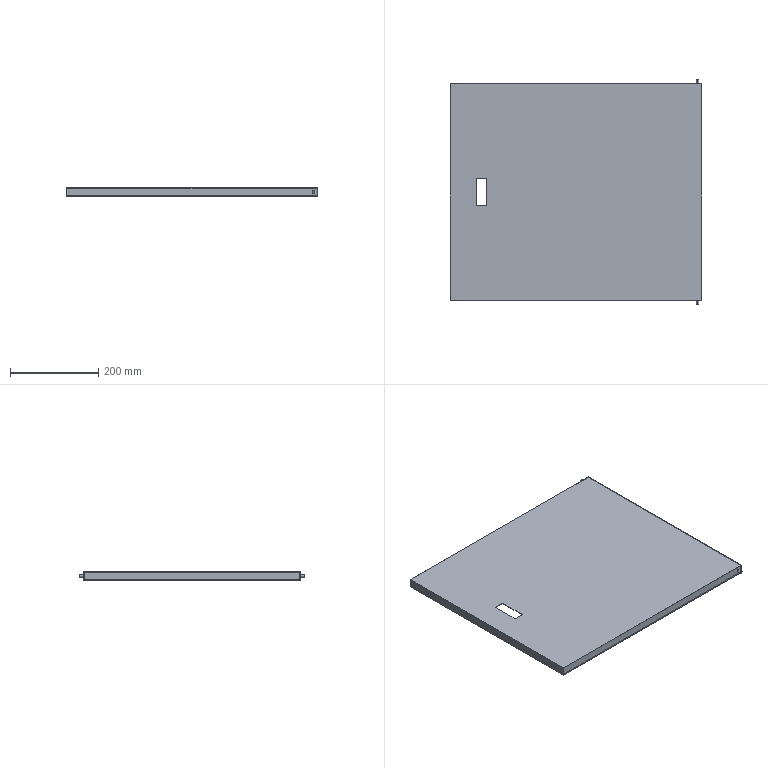Part | SolidWorks | features ICE 4, Extrusion 1, Shell 1 | 1 solid | 26 faces | box 570 x 510 x 20 mm | volume 346646 mm3 | plane 22 | cylinder 4 | commonest cylinder face diameters 6 x4
STEP:
#1=CARTESIAN_POINT('',(275.,-255.,7.));
#2=VERTEX_POINT('',#1);
#3=CARTESIAN_POINT('',(275.,-255.,13.));
#4=VERTEX_POINT('',#3);
#5=CARTESIAN_POINT('',(275.,-255.,10.));
#6=DIRECTION('',(0.,-1.,0.));
#7=DIRECTION('',(0.,0.,-1.));
#8=AXIS2_PLACEMENT_3D('',#5,#6,#7);
#9=CIRCLE('',#8,3.);
#10=EDGE_CURVE('',#2,#4,#9,.T.);
#11=ORIENTED_EDGE('',*,*,#10,.F.);
#12=CARTESIAN_POINT('',(275.,-245.,7.));
#13=VERTEX_POINT('',#12);
#14=CARTESIAN_POINT('',(275.,-255.,7.));
#15=DIRECTION('',(0.,1.,0.));
#16=VECTOR('',#15,1000.);
#17=LINE('',#14,#16);
#18=EDGE_CURVE('',#2,#13,#17,.T.);
#19=ORIENTED_EDGE('',*,*,#18,.T.);
#20=CARTESIAN_POINT('',(275.,-245.,13.));
#21=VERTEX_POINT('',#20);
#22=CARTESIAN_POINT('',(275.,-245.,10.));
#23=DIRECTION('',(0.,-1.,0.));
#24=DIRECTION('',(0.,0.,1.));
#25=AXIS2_PLACEMENT_3D('',#22,#23,#24);
#26=CIRCLE('',#25,3.);
#27=EDGE_CURVE('',#13,#21,#26,.T.);
#28=ORIENTED_EDGE('',*,*,#27,.T.);
#29=CARTESIAN_POINT('',(275.,-255.,13.));
#30=DIRECTION('',(0.,1.,0.));
#31=VECTOR('',#30,1000.);
#32=LINE('',#29,#31);
#33=EDGE_CURVE('',#4,#21,#32,.T.);
#34=ORIENTED_EDGE('',*,*,#33,.F.);
#35=EDGE_LOOP('',(#11,#19,#28,#34));
#36=FACE_OUTER_BOUND('',#35,.T.);
#37=CARTESIAN_POINT('',(275.,-255.,10.));
#38=DIRECTION('',(0.,1.,0.));
#39=DIRECTION('',(0.,0.,1.));
#40=AXIS2_PLACEMENT_3D('',#37,#38,#39);
#41=CYLINDRICAL_SURFACE('',#40,3.);
#42=ADVANCED_FACE('',(#36),#41,.T.);
#43=CARTESIAN_POINT('',(275.,255.,13.));
#44=VERTEX_POINT('',#43);
#45=CARTESIAN_POINT('',(275.,255.,7.));
#46=VERTEX_POINT('',#45);
#47=CARTESIAN_POINT('',(275.,255.,10.));
#48=DIRECTION('',(0.,1.,0.));
#49=DIRECTION('',(0.,0.,1.));
#50=AXIS2_PLACEMENT_3D('',#47,#48,#49);
#51=CIRCLE('',#50,3.);
#52=EDGE_CURVE('',#44,#46,#51,.T.);
#53=ORIENTED_EDGE('',*,*,#52,.F.);
#54=CARTESIAN_POINT('',(275.,245.,13.));
#55=VERTEX_POINT('',#54);
#56=CARTESIAN_POINT('',(275.,255.,13.));
#57=DIRECTION('',(0.,-1.,0.));
#58=VECTOR('',#57,1000.);
#59=LINE('',#56,#58);
#60=EDGE_CURVE('',#44,#55,#59,.T.);
#61=ORIENTED_EDGE('',*,*,#60,.T.);
#62=CARTESIAN_POINT('',(275.,245.,7.));
#63=VERTEX_POINT('',#62);
#64=CARTESIAN_POINT('',(275.,245.,10.));
#65=DIRECTION('',(0.,1.,0.));
#66=DIRECTION('',(0.,0.,-1.));
#67=AXIS2_PLACEMENT_3D('',#64,#65,#66);
#68=CIRCLE('',#67,3.);
#69=EDGE_CURVE('',#55,#63,#68,.T.);
#70=ORIENTED_EDGE('',*,*,#69,.T.);
#71=CARTESIAN_POINT('',(275.,255.,7.));
#72=DIRECTION('',(0.,-1.,0.));
#73=VECTOR('',#72,1000.);
#74=LINE('',#71,#73);
#75=EDGE_CURVE('',#46,#63,#74,.T.);
#76=ORIENTED_EDGE('',*,*,#75,.F.);
#77=EDGE_LOOP('',(#53,#61,#70,#76));
#78=FACE_OUTER_BOUND('',#77,.T.);
#79=CARTESIAN_POINT('',(275.,255.,10.));
#80=DIRECTION('',(0.,-1.,0.));
#81=DIRECTION('',(0.,0.,-1.));
#82=AXIS2_PLACEMENT_3D('',#79,#80,#81);
#83=CYLINDRICAL_SURFACE('',#82,3.);
#84=ADVANCED_FACE('',(#78),#83,.T.);
#85=CARTESIAN_POINT('',(-285.,-245.,0.));
#86=VERTEX_POINT('',#85);
#87=CARTESIAN_POINT('',(285.,-245.,0.));
#88=VERTEX_POINT('',#87);
#89=CARTESIAN_POINT('',(-285.,-245.,0.));
#90=DIRECTION('',(1.,0.,0.));
#91=VECTOR('',#90,1000.);
#92=LINE('',#89,#91);
#93=EDGE_CURVE('',#86,#88,#92,.T.);
#94=ORIENTED_EDGE('',*,*,#93,.T.);
#95=CARTESIAN_POINT('',(285.,-245.,20.));
#96=VERTEX_POINT('',#95);
#97=CARTESIAN_POINT('',(285.,-245.,20.));
#98=DIRECTION('',(0.,0.,-1.));
#99=VECTOR('',#98,1000.);
#100=LINE('',#97,#99);
#101=EDGE_CURVE('',#96,#88,#100,.T.);
#102=ORIENTED_EDGE('',*,*,#101,.F.);
#103=CARTESIAN_POINT('',(-285.,-245.,20.));
#104=VERTEX_POINT('',#103);
#105=CARTESIAN_POINT('',(-285.,-245.,20.));
#106=DIRECTION('',(1.,0.,0.));
#107=VECTOR('',#106,1000.);
#108=LINE('',#105,#107);
#109=EDGE_CURVE('',#104,#96,#108,.T.);
#110=ORIENTED_EDGE('',*,*,#109,.F.);
#111=CARTESIAN_POINT('',(-285.,-245.,20.));
#112=DIRECTION('',(0.,0.,-1.));
#113=VECTOR('',#112,1000.);
#114=LINE('',#111,#113);
#115=EDGE_CURVE('',#104,#86,#114,.T.);
#116=ORIENTED_EDGE('',*,*,#115,.T.);
#117=EDGE_LOOP('',(#94,#102,#110,#116));
#118=FACE_OUTER_BOUND('',#117,.T.);
#119=CARTESIAN_POINT('',(275.,-245.,10.));
#120=DIRECTION('',(0.,-1.,0.));
#121=DIRECTION('',(0.,0.,1.));
#122=AXIS2_PLACEMENT_3D('',#119,#120,#121);
#123=CIRCLE('',#122,3.);
#124=EDGE_CURVE('',#21,#13,#123,.T.);
#125=ORIENTED_EDGE('',*,*,#124,.F.);
#126=ORIENTED_EDGE('',*,*,#27,.F.);
#127=EDGE_LOOP('',(#125,#126));
#128=FACE_BOUND('',#127,.T.);
#129=CARTESIAN_POINT('',(-285.,-245.,20.));
#130=DIRECTION('',(0.,1.,0.));
#131=DIRECTION('',(0.,0.,1.));
#132=AXIS2_PLACEMENT_3D('',#129,#130,#131);
#133=PLANE('',#132);
#134=ADVANCED_FACE('',(#118,#128),#133,.F.);
#135=CARTESIAN_POINT('',(285.,245.,0.));
#136=VERTEX_POINT('',#135);
#137=CARTESIAN_POINT('',(-285.,245.,0.));
#138=VERTEX_POINT('',#137);
#139=CARTESIAN_POINT('',(-285.,245.,0.));
#140=DIRECTION('',(-1.,0.,0.));
#141=VECTOR('',#140,1000.);
#142=LINE('',#139,#141);
#143=EDGE_CURVE('',#136,#138,#142,.T.);
#144=ORIENTED_EDGE('',*,*,#143,.T.);
#145=CARTESIAN_POINT('',(-285.,245.,20.));
#146=VERTEX_POINT('',#145);
#147=CARTESIAN_POINT('',(-285.,245.,20.));
#148=DIRECTION('',(0.,0.,-1.));
#149=VECTOR('',#148,1000.);
#150=LINE('',#147,#149);
#151=EDGE_CURVE('',#146,#138,#150,.T.);
#152=ORIENTED_EDGE('',*,*,#151,.F.);
#153=CARTESIAN_POINT('',(285.,245.,20.));
#154=VERTEX_POINT('',#153);
#155=CARTESIAN_POINT('',(-285.,245.,20.));
#156=DIRECTION('',(-1.,0.,0.));
#157=VECTOR('',#156,1000.);
#158=LINE('',#155,#157);
#159=EDGE_CURVE('',#154,#146,#158,.T.);
#160=ORIENTED_EDGE('',*,*,#159,.F.);
#161=CARTESIAN_POINT('',(285.,245.,20.));
#162=DIRECTION('',(0.,0.,-1.));
#163=VECTOR('',#162,1000.);
#164=LINE('',#161,#163);
#165=EDGE_CURVE('',#154,#136,#164,.T.);
#166=ORIENTED_EDGE('',*,*,#165,.T.);
#167=EDGE_LOOP('',(#144,#152,#160,#166));
#168=FACE_OUTER_BOUND('',#167,.T.);
#169=CARTESIAN_POINT('',(275.,245.,10.));
#170=DIRECTION('',(0.,1.,0.));
#171=DIRECTION('',(0.,0.,-1.));
#172=AXIS2_PLACEMENT_3D('',#169,#170,#171);
#173=CIRCLE('',#172,3.);
#174=EDGE_CURVE('',#63,#55,#173,.T.);
#175=ORIENTED_EDGE('',*,*,#174,.F.);
#176=ORIENTED_EDGE('',*,*,#69,.F.);
#177=EDGE_LOOP('',(#175,#176));
#178=FACE_BOUND('',#177,.T.);
#179=CARTESIAN_POINT('',(-285.,245.,20.));
#180=DIRECTION('',(0.,-1.,0.));
#181=DIRECTION('',(0.,0.,-1.));
#182=AXIS2_PLACEMENT_3D('',#179,#180,#181);
#183=PLANE('',#182);
#184=ADVANCED_FACE('',(#168,#178),#183,.F.);
#185=CARTESIAN_POINT('',(285.,245.,0.));
#186=DIRECTION('',(0.,1.,0.));
#187=VECTOR('',#186,1000.);
#188=LINE('',#185,#187);
#189=EDGE_CURVE('',#88,#136,#188,.T.);
#190=ORIENTED_EDGE('',*,*,#189,.T.);
#191=ORIENTED_EDGE('',*,*,#165,.F.);
#192=CARTESIAN_POINT('',(285.,245.,20.));
#193=DIRECTION('',(0.,1.,0.));
#194=VECTOR('',#193,1000.);
#195=LINE('',#192,#194);
#196=EDGE_CURVE('',#96,#154,#195,.T.);
#197=ORIENTED_EDGE('',*,*,#196,.F.);
#198=ORIENTED_EDGE('',*,*,#101,.T.);
#199=EDGE_LOOP('',(#190,#191,#197,#198));
#200=FACE_OUTER_BOUND('',#199,.T.);
#201=CARTESIAN_POINT('',(285.,245.,20.));
#202=DIRECTION('',(-1.,0.,0.));
#203=DIRECTION('',(0.,0.,1.));
#204=AXIS2_PLACEMENT_3D('',#201,#202,#203);
#205=PLANE('',#204);
#206=ADVANCED_FACE('',(#200),#205,.F.);
#207=CARTESIAN_POINT('',(-285.,245.,0.));
#208=DIRECTION('',(0.,-1.,0.));
#209=VECTOR('',#208,1000.);
#210=LINE('',#207,#209);
#211=EDGE_CURVE('',#138,#86,#210,.T.);
#212=ORIENTED_EDGE('',*,*,#211,.T.);
#213=ORIENTED_EDGE('',*,*,#115,.F.);
#214=CARTESIAN_POINT('',(-285.,245.,20.));
#215=DIRECTION('',(0.,-1.,0.));
#216=VECTOR('',#215,1000.);
#217=LINE('',#214,#216);
#218=EDGE_CURVE('',#146,#104,#217,.T.);
#219=ORIENTED_EDGE('',*,*,#218,.F.);
#220=ORIENTED_EDGE('',*,*,#151,.T.);
#221=EDGE_LOOP('',(#212,#213,#219,#220));
#222=FACE_OUTER_BOUND('',#221,.T.);
#223=CARTESIAN_POINT('',(-285.,245.,20.));
#224=DIRECTION('',(1.,0.,0.));
#225=DIRECTION('',(0.,0.,-1.));
#226=AXIS2_PLACEMENT_3D('',#223,#224,#225);
#227=PLANE('',#226);
#228=ADVANCED_FACE('',(#222),#227,.F.);
#229=CARTESIAN_POINT('',(-202.,-31.5,20.));
#230=VERTEX_POINT('',#229);
#231=CARTESIAN_POINT('',(-202.,31.5,20.));
#232=VERTEX_POINT('',#231);
#233=CARTESIAN_POINT('',(-202.,-31.5,20.));
#234=DIRECTION('',(0.,1.,0.));
#235=VECTOR('',#234,1000.);
#236=LINE('',#233,#235);
#237=EDGE_CURVE('',#230,#232,#236,.T.);
#238=ORIENTED_EDGE('',*,*,#237,.F.);
#239=CARTESIAN_POINT('',(-225.,-31.5,20.));
#240=VERTEX_POINT('',#239);
#241=CARTESIAN_POINT('',(-225.,-31.5,20.));
#242=DIRECTION('',(1.,0.,0.));
#243=VECTOR('',#242,1000.);
#244=LINE('',#241,#243);
#245=EDGE_CURVE('',#240,#230,#244,.T.);
#246=ORIENTED_EDGE('',*,*,#245,.F.);
#247=CARTESIAN_POINT('',(-225.,31.5,20.));
#248=VERTEX_POINT('',#247);
#249=CARTESIAN_POINT('',(-225.,-31.5,20.));
#250=DIRECTION('',(0.,-1.,0.));
#251=VECTOR('',#250,1000.);
#252=LINE('',#249,#251);
#253=EDGE_CURVE('',#248,#240,#252,.T.);
#254=ORIENTED_EDGE('',*,*,#253,.F.);
#255=CARTESIAN_POINT('',(-225.,31.5,20.));
#256=DIRECTION('',(-1.,0.,0.));
#257=VECTOR('',#256,1000.);
#258=LINE('',#255,#257);
#259=EDGE_CURVE('',#232,#248,#258,.T.);
#260=ORIENTED_EDGE('',*,*,#259,.F.);
#261=EDGE_LOOP('',(#238,#246,#254,#260));
#262=FACE_BOUND('',#261,.T.);
#263=ORIENTED_EDGE('',*,*,#196,.T.);
#264=ORIENTED_EDGE('',*,*,#159,.T.);
#265=ORIENTED_EDGE('',*,*,#218,.T.);
#266=ORIENTED_EDGE('',*,*,#109,.T.);
#267=EDGE_LOOP('',(#263,#264,#265,#266));
#268=FACE_OUTER_BOUND('',#267,.T.);
#269=CARTESIAN_POINT('',(285.,-245.,20.));
#270=DIRECTION('',(0.,0.,1.));
#271=DIRECTION('',(1.,0.,0.));
#272=AXIS2_PLACEMENT_3D('',#269,#270,#271);
#273=PLANE('',#272);
#274=ADVANCED_FACE('',(#262,#268),#273,.T.);
#275=ORIENTED_EDGE('',*,*,#189,.F.);
#276=ORIENTED_EDGE('',*,*,#93,.F.);
#277=ORIENTED_EDGE('',*,*,#211,.F.);
#278=ORIENTED_EDGE('',*,*,#143,.F.);
#279=EDGE_LOOP('',(#275,#276,#277,#278));
#280=FACE_OUTER_BOUND('',#279,.T.);
#281=CARTESIAN_POINT('',(-275.,235.,0.));
#282=VERTEX_POINT('',#281);
#283=CARTESIAN_POINT('',(275.,235.,0.));
#284=VERTEX_POINT('',#283);
#285=CARTESIAN_POINT('',(275.,235.,0.));
#286=DIRECTION('',(1.,0.,0.));
#287=VECTOR('',#286,1000.);
#288=LINE('',#285,#287);
#289=EDGE_CURVE('',#282,#284,#288,.T.);
#290=ORIENTED_EDGE('',*,*,#289,.F.);
#291=CARTESIAN_POINT('',(-275.,-235.,0.));
#292=VERTEX_POINT('',#291);
#293=CARTESIAN_POINT('',(-275.,235.,0.));
#294=DIRECTION('',(0.,1.,0.));
#295=VECTOR('',#294,1000.);
#296=LINE('',#293,#295);
#297=EDGE_CURVE('',#292,#282,#296,.T.);
#298=ORIENTED_EDGE('',*,*,#297,.F.);
#299=CARTESIAN_POINT('',(275.,-235.,0.));
#300=VERTEX_POINT('',#299);
#301=CARTESIAN_POINT('',(275.,-235.,0.));
#302=DIRECTION('',(-1.,0.,0.));
#303=VECTOR('',#302,1000.);
#304=LINE('',#301,#303);
#305=EDGE_CURVE('',#300,#292,#304,.T.);
#306=ORIENTED_EDGE('',*,*,#305,.F.);
#307=CARTESIAN_POINT('',(275.,235.,0.));
#308=DIRECTION('',(0.,-1.,0.));
#309=VECTOR('',#308,1000.);
#310=LINE('',#307,#309);
#311=EDGE_CURVE('',#284,#300,#310,.T.);
#312=ORIENTED_EDGE('',*,*,#311,.F.);
#313=EDGE_LOOP('',(#290,#298,#306,#312));
#314=FACE_BOUND('',#313,.T.);
#315=CARTESIAN_POINT('',(285.,-245.,0.));
#316=DIRECTION('',(0.,0.,1.));
#317=DIRECTION('',(1.,0.,0.));
#318=AXIS2_PLACEMENT_3D('',#315,#316,#317);
#319=PLANE('',#318);
#320=ADVANCED_FACE('',(#280,#314),#319,.F.);
#321=CARTESIAN_POINT('',(284.,244.,1.5));
#322=VERTEX_POINT('',#321);
#323=CARTESIAN_POINT('',(284.,-244.,1.5));
#324=VERTEX_POINT('',#323);
#325=CARTESIAN_POINT('',(284.,245.,1.5));
#326=DIRECTION('',(0.,-1.,0.));
#327=VECTOR('',#326,1000.);
#328=LINE('',#325,#327);
#329=EDGE_CURVE('',#322,#324,#328,.T.);
#330=ORIENTED_EDGE('',*,*,#329,.F.);
#331=CARTESIAN_POINT('',(-284.,244.,1.5));
#332=VERTEX_POINT('',#331);
#333=CARTESIAN_POINT('',(-285.,244.,1.5));
#334=DIRECTION('',(1.,0.,0.));
#335=VECTOR('',#334,1000.);
#336=LINE('',#333,#335);
#337=EDGE_CURVE('',#332,#322,#336,.T.);
#338=ORIENTED_EDGE('',*,*,#337,.F.);
#339=CARTESIAN_POINT('',(-284.,-244.,1.5));
#340=VERTEX_POINT('',#339);
#341=CARTESIAN_POINT('',(-284.,245.,1.5));
#342=DIRECTION('',(0.,1.,0.));
#343=VECTOR('',#342,1000.);
#344=LINE('',#341,#343);
#345=EDGE_CURVE('',#340,#332,#344,.T.);
#346=ORIENTED_EDGE('',*,*,#345,.F.);
#347=CARTESIAN_POINT('',(-285.,-244.,1.5));
#348=DIRECTION('',(-1.,0.,0.));
#349=VECTOR('',#348,1000.);
#350=LINE('',#347,#349);
#351=EDGE_CURVE('',#324,#340,#350,.T.);
#352=ORIENTED_EDGE('',*,*,#351,.F.);
#353=EDGE_LOOP('',(#330,#338,#346,#352));
#354=FACE_OUTER_BOUND('',#353,.T.);
#355=CARTESIAN_POINT('',(-275.,-235.,1.5));
#356=VERTEX_POINT('',#355);
#357=CARTESIAN_POINT('',(-275.,235.,1.5));
#358=VERTEX_POINT('',#357);
#359=CARTESIAN_POINT('',(-275.,235.,1.5));
#360=DIRECTION('',(0.,1.,0.));
#361=VECTOR('',#360,1000.);
#362=LINE('',#359,#361);
#363=EDGE_CURVE('',#356,#358,#362,.T.);
#364=ORIENTED_EDGE('',*,*,#363,.T.);
#365=CARTESIAN_POINT('',(275.,235.,1.5));
#366=VERTEX_POINT('',#365);
#367=CARTESIAN_POINT('',(275.,235.,1.5));
#368=DIRECTION('',(1.,0.,0.));
#369=VECTOR('',#368,1000.);
#370=LINE('',#367,#369);
#371=EDGE_CURVE('',#358,#366,#370,.T.);
#372=ORIENTED_EDGE('',*,*,#371,.T.);
#373=CARTESIAN_POINT('',(275.,-235.,1.5));
#374=VERTEX_POINT('',#373);
#375=CARTESIAN_POINT('',(275.,235.,1.5));
#376=DIRECTION('',(0.,-1.,0.));
#377=VECTOR('',#376,1000.);
#378=LINE('',#375,#377);
#379=EDGE_CURVE('',#366,#374,#378,.T.);
#380=ORIENTED_EDGE('',*,*,#379,.T.);
#381=CARTESIAN_POINT('',(275.,-235.,1.5));
#382=DIRECTION('',(-1.,0.,0.));
#383=VECTOR('',#382,1000.);
#384=LINE('',#381,#383);
#385=EDGE_CURVE('',#374,#356,#384,.T.);
#386=ORIENTED_EDGE('',*,*,#385,.T.);
#387=EDGE_LOOP('',(#364,#372,#380,#386));
#388=FACE_BOUND('',#387,.T.);
#389=CARTESIAN_POINT('',(285.,-245.,1.5));
#390=DIRECTION('',(0.,0.,-1.));
#391=DIRECTION('',(-1.,0.,0.));
#392=AXIS2_PLACEMENT_3D('',#389,#390,#391);
#393=PLANE('',#392);
#394=ADVANCED_FACE('',(#354,#388),#393,.F.);
#395=ORIENTED_EDGE('',*,*,#289,.T.);
#396=CARTESIAN_POINT('',(275.,235.,1.5));
#397=DIRECTION('',(0.,0.,-1.));
#398=VECTOR('',#397,1000.);
#399=LINE('',#396,#398);
#400=EDGE_CURVE('',#366,#284,#399,.T.);
#401=ORIENTED_EDGE('',*,*,#400,.F.);
#402=ORIENTED_EDGE('',*,*,#371,.F.);
#403=CARTESIAN_POINT('',(-275.,235.,1.5));
#404=DIRECTION('',(0.,0.,-1.));
#405=VECTOR('',#404,1000.);
#406=LINE('',#403,#405);
#407=EDGE_CURVE('',#358,#282,#406,.T.);
#408=ORIENTED_EDGE('',*,*,#407,.T.);
#409=EDGE_LOOP('',(#395,#401,#402,#408));
#410=FACE_OUTER_BOUND('',#409,.T.);
#411=CARTESIAN_POINT('',(275.,235.,1.5));
#412=DIRECTION('',(0.,1.,0.));
#413=DIRECTION('',(0.,0.,1.));
#414=AXIS2_PLACEMENT_3D('',#411,#412,#413);
#415=PLANE('',#414);
#416=ADVANCED_FACE('',(#410),#415,.F.);
#417=ORIENTED_EDGE('',*,*,#297,.T.);
#418=ORIENTED_EDGE('',*,*,#407,.F.);
#419=ORIENTED_EDGE('',*,*,#363,.F.);
#420=CARTESIAN_POINT('',(-275.,-235.,1.5));
#421=DIRECTION('',(0.,0.,-1.));
#422=VECTOR('',#421,1000.);
#423=LINE('',#420,#422);
#424=EDGE_CURVE('',#356,#292,#423,.T.);
#425=ORIENTED_EDGE('',*,*,#424,.T.);
#426=EDGE_LOOP('',(#417,#418,#419,#425));
#427=FACE_OUTER_BOUND('',#426,.T.);
#428=CARTESIAN_POINT('',(-275.,235.,1.5));
#429=DIRECTION('',(-1.,0.,0.));
#430=DIRECTION('',(0.,-1.,0.));
#431=AXIS2_PLACEMENT_3D('',#428,#429,#430);
#432=PLANE('',#431);
#433=ADVANCED_FACE('',(#427),#432,.F.);
#434=ORIENTED_EDGE('',*,*,#305,.T.);
#435=ORIENTED_EDGE('',*,*,#424,.F.);
#436=ORIENTED_EDGE('',*,*,#385,.F.);
#437=CARTESIAN_POINT('',(275.,-235.,1.5));
#438=DIRECTION('',(0.,0.,-1.));
#439=VECTOR('',#438,1000.);
#440=LINE('',#437,#439);
#441=EDGE_CURVE('',#374,#300,#440,.T.);
#442=ORIENTED_EDGE('',*,*,#441,.T.);
#443=EDGE_LOOP('',(#434,#435,#436,#442));
#444=FACE_OUTER_BOUND('',#443,.T.);
#445=CARTESIAN_POINT('',(275.,-235.,1.5));
#446=DIRECTION('',(0.,-1.,0.));
#447=DIRECTION('',(1.,0.,0.));
#448=AXIS2_PLACEMENT_3D('',#445,#446,#447);
#449=PLANE('',#448);
#450=ADVANCED_FACE('',(#444),#449,.F.);
#451=ORIENTED_EDGE('',*,*,#311,.T.);
#452=ORIENTED_EDGE('',*,*,#441,.F.);
#453=ORIENTED_EDGE('',*,*,#379,.F.);
#454=ORIENTED_EDGE('',*,*,#400,.T.);
#455=EDGE_LOOP('',(#451,#452,#453,#454));
#456=FACE_OUTER_BOUND('',#455,.T.);
#457=CARTESIAN_POINT('',(275.,235.,1.5));
#458=DIRECTION('',(1.,0.,0.));
#459=DIRECTION('',(0.,1.,0.));
#460=AXIS2_PLACEMENT_3D('',#457,#458,#459);
#461=PLANE('',#460);
#462=ADVANCED_FACE('',(#456),#461,.F.);
#463=CARTESIAN_POINT('',(-225.,-31.5,19.));
#464=VERTEX_POINT('',#463);
#465=CARTESIAN_POINT('',(-202.,-31.5,19.));
#466=VERTEX_POINT('',#465);
#467=CARTESIAN_POINT('',(285.,-31.5,19.));
#468=DIRECTION('',(1.,0.,0.));
#469=VECTOR('',#468,1000.);
#470=LINE('',#467,#469);
#471=EDGE_CURVE('',#464,#466,#470,.T.);
#472=ORIENTED_EDGE('',*,*,#471,.T.);
#473=CARTESIAN_POINT('',(-202.,31.5,19.));
#474=VERTEX_POINT('',#473);
#475=CARTESIAN_POINT('',(-202.,-245.,19.));
#476=DIRECTION('',(0.,1.,0.));
#477=VECTOR('',#476,1000.);
#478=LINE('',#475,#477);
#479=EDGE_CURVE('',#466,#474,#478,.T.);
#480=ORIENTED_EDGE('',*,*,#479,.T.);
#481=CARTESIAN_POINT('',(-225.,31.5,19.));
#482=VERTEX_POINT('',#481);
#483=CARTESIAN_POINT('',(285.,31.5,19.));
#484=DIRECTION('',(-1.,0.,0.));
#485=VECTOR('',#484,1000.);
#486=LINE('',#483,#485);
#487=EDGE_CURVE('',#474,#482,#486,.T.);
#488=ORIENTED_EDGE('',*,*,#487,.T.);
#489=CARTESIAN_POINT('',(-225.,-245.,19.));
#490=DIRECTION('',(0.,-1.,0.));
#491=VECTOR('',#490,1000.);
#492=LINE('',#489,#491);
#493=EDGE_CURVE('',#482,#464,#492,.T.);
#494=ORIENTED_EDGE('',*,*,#493,.T.);
#495=EDGE_LOOP('',(#472,#480,#488,#494));
#496=FACE_BOUND('',#495,.T.);
#497=CARTESIAN_POINT('',(284.,-244.,19.));
#498=VERTEX_POINT('',#497);
#499=CARTESIAN_POINT('',(284.,244.,19.));
#500=VERTEX_POINT('',#499);
#501=CARTESIAN_POINT('',(284.,245.,19.));
#502=DIRECTION('',(0.,1.,0.));
#503=VECTOR('',#502,1000.);
#504=LINE('',#501,#503);
#505=EDGE_CURVE('',#498,#500,#504,.T.);
#506=ORIENTED_EDGE('',*,*,#505,.F.);
#507=CARTESIAN_POINT('',(-284.,-244.,19.));
#508=VERTEX_POINT('',#507);
#509=CARTESIAN_POINT('',(-285.,-244.,19.));
#510=DIRECTION('',(1.,0.,0.));
#511=VECTOR('',#510,1000.);
#512=LINE('',#509,#511);
#513=EDGE_CURVE('',#508,#498,#512,.T.);
#514=ORIENTED_EDGE('',*,*,#513,.F.);
#515=CARTESIAN_POINT('',(-284.,244.,19.));
#516=VERTEX_POINT('',#515);
#517=CARTESIAN_POINT('',(-284.,245.,19.));
#518=DIRECTION('',(0.,-1.,0.));
#519=VECTOR('',#518,1000.);
#520=LINE('',#517,#519);
#521=EDGE_CURVE('',#516,#508,#520,.T.);
#522=ORIENTED_EDGE('',*,*,#521,.F.);
#523=CARTESIAN_POINT('',(-285.,244.,19.));
#524=DIRECTION('',(-1.,0.,0.));
#525=VECTOR('',#524,1000.);
#526=LINE('',#523,#525);
#527=EDGE_CURVE('',#500,#516,#526,.T.);
#528=ORIENTED_EDGE('',*,*,#527,.F.);
#529=EDGE_LOOP('',(#506,#514,#522,#528));
#530=FACE_OUTER_BOUND('',#529,.T.);
#531=CARTESIAN_POINT('',(285.,-245.,19.));
#532=DIRECTION('',(0.,0.,1.));
#533=DIRECTION('',(1.,0.,0.));
#534=AXIS2_PLACEMENT_3D('',#531,#532,#533);
#535=PLANE('',#534);
#536=ADVANCED_FACE('',(#496,#530),#535,.F.);
#537=CARTESIAN_POINT('',(284.,-244.,20.));
#538=DIRECTION('',(0.,0.,-1.));
#539=VECTOR('',#538,1000.);
#540=LINE('',#537,#539);
#541=EDGE_CURVE('',#498,#324,#540,.T.);
#542=ORIENTED_EDGE('',*,*,#541,.T.);
#543=ORIENTED_EDGE('',*,*,#351,.T.);
#544=CARTESIAN_POINT('',(-284.,-244.,20.));
#545=DIRECTION('',(0.,0.,-1.));
#546=VECTOR('',#545,1000.);
#547=LINE('',#544,#546);
#548=EDGE_CURVE('',#508,#340,#547,.T.);
#549=ORIENTED_EDGE('',*,*,#548,.F.);
#550=ORIENTED_EDGE('',*,*,#513,.T.);
#551=EDGE_LOOP('',(#542,#543,#549,#550));
#552=FACE_OUTER_BOUND('',#551,.T.);
#553=CARTESIAN_POINT('',(-285.,-244.,20.));
#554=DIRECTION('',(0.,1.,0.));
#555=DIRECTION('',(0.,0.,1.));
#556=AXIS2_PLACEMENT_3D('',#553,#554,#555);
#557=PLANE('',#556);
#558=ADVANCED_FACE('',(#552),#557,.T.);
#559=ORIENTED_EDGE('',*,*,#548,.T.);
#560=ORIENTED_EDGE('',*,*,#345,.T.);
#561=CARTESIAN_POINT('',(-284.,244.,20.));
#562=DIRECTION('',(0.,0.,-1.));
#563=VECTOR('',#562,1000.);
#564=LINE('',#561,#563);
#565=EDGE_CURVE('',#516,#332,#564,.T.);
#566=ORIENTED_EDGE('',*,*,#565,.F.);
#567=ORIENTED_EDGE('',*,*,#521,.T.);
#568=EDGE_LOOP('',(#559,#560,#566,#567));
#569=FACE_OUTER_BOUND('',#568,.T.);
#570=CARTESIAN_POINT('',(-284.,245.,20.));
#571=DIRECTION('',(1.,0.,0.));
#572=DIRECTION('',(0.,0.,-1.));
#573=AXIS2_PLACEMENT_3D('',#570,#571,#572);
#574=PLANE('',#573);
#575=ADVANCED_FACE('',(#569),#574,.T.);
#576=ORIENTED_EDGE('',*,*,#565,.T.);
#577=ORIENTED_EDGE('',*,*,#337,.T.);
#578=CARTESIAN_POINT('',(284.,244.,20.));
#579=DIRECTION('',(0.,0.,-1.));
#580=VECTOR('',#579,1000.);
#581=LINE('',#578,#580);
#582=EDGE_CURVE('',#500,#322,#581,.T.);
#583=ORIENTED_EDGE('',*,*,#582,.F.);
#584=ORIENTED_EDGE('',*,*,#527,.T.);
#585=EDGE_LOOP('',(#576,#577,#583,#584));
#586=FACE_OUTER_BOUND('',#585,.T.);
#587=CARTESIAN_POINT('',(-285.,244.,20.));
#588=DIRECTION('',(0.,-1.,0.));
#589=DIRECTION('',(0.,0.,-1.));
#590=AXIS2_PLACEMENT_3D('',#587,#588,#589);
#591=PLANE('',#590);
#592=ADVANCED_FACE('',(#586),#591,.T.);
#593=ORIENTED_EDGE('',*,*,#582,.T.);
#594=ORIENTED_EDGE('',*,*,#329,.T.);
#595=ORIENTED_EDGE('',*,*,#541,.F.);
#596=ORIENTED_EDGE('',*,*,#505,.T.);
#597=EDGE_LOOP('',(#593,#594,#595,#596));
#598=FACE_OUTER_BOUND('',#597,.T.);
#599=CARTESIAN_POINT('',(284.,245.,20.));
#600=DIRECTION('',(-1.,0.,0.));
#601=DIRECTION('',(0.,0.,1.));
#602=AXIS2_PLACEMENT_3D('',#599,#600,#601);
#603=PLANE('',#602);
#604=ADVANCED_FACE('',(#598),#603,.T.);
#605=ORIENTED_EDGE('',*,*,#60,.F.);
#606=CARTESIAN_POINT('',(275.,255.,10.));
#607=DIRECTION('',(0.,1.,0.));
#608=DIRECTION('',(0.,0.,1.));
#609=AXIS2_PLACEMENT_3D('',#606,#607,#608);
#610=CIRCLE('',#609,3.);
#611=EDGE_CURVE('',#46,#44,#610,.T.);
#612=ORIENTED_EDGE('',*,*,#611,.F.);
#613=ORIENTED_EDGE('',*,*,#75,.T.);
#614=ORIENTED_EDGE('',*,*,#174,.T.);
#615=EDGE_LOOP('',(#605,#612,#613,#614));
#616=FACE_OUTER_BOUND('',#615,.T.);
#617=CARTESIAN_POINT('',(275.,255.,10.));
#618=DIRECTION('',(0.,-1.,0.));
#619=DIRECTION('',(0.,0.,-1.));
#620=AXIS2_PLACEMENT_3D('',#617,#618,#619);
#621=CYLINDRICAL_SURFACE('',#620,3.);
#622=ADVANCED_FACE('',(#616),#621,.T.);
#623=ORIENTED_EDGE('',*,*,#611,.T.);
#624=ORIENTED_EDGE('',*,*,#52,.T.);
#625=EDGE_LOOP('',(#623,#624));
#626=FACE_OUTER_BOUND('',#625,.T.);
#627=CARTESIAN_POINT('',(275.,255.,10.));
#628=DIRECTION('',(0.,1.,0.));
#629=DIRECTION('',(0.,0.,1.));
#630=AXIS2_PLACEMENT_3D('',#627,#628,#629);
#631=PLANE('',#630);
#632=ADVANCED_FACE('',(#626),#631,.T.);
#633=ORIENTED_EDGE('',*,*,#18,.F.);
#634=CARTESIAN_POINT('',(275.,-255.,10.));
#635=DIRECTION('',(0.,-1.,0.));
#636=DIRECTION('',(0.,0.,-1.));
#637=AXIS2_PLACEMENT_3D('',#634,#635,#636);
#638=CIRCLE('',#637,3.);
#639=EDGE_CURVE('',#4,#2,#638,.T.);
#640=ORIENTED_EDGE('',*,*,#639,.F.);
#641=ORIENTED_EDGE('',*,*,#33,.T.);
#642=ORIENTED_EDGE('',*,*,#124,.T.);
#643=EDGE_LOOP('',(#633,#640,#641,#642));
#644=FACE_OUTER_BOUND('',#643,.T.);
#645=CARTESIAN_POINT('',(275.,-255.,10.));
#646=DIRECTION('',(0.,1.,0.));
#647=DIRECTION('',(0.,0.,1.));
#648=AXIS2_PLACEMENT_3D('',#645,#646,#647);
#649=CYLINDRICAL_SURFACE('',#648,3.);
#650=ADVANCED_FACE('',(#644),#649,.T.);
#651=ORIENTED_EDGE('',*,*,#639,.T.);
#652=ORIENTED_EDGE('',*,*,#10,.T.);
#653=EDGE_LOOP('',(#651,#652));
#654=FACE_OUTER_BOUND('',#653,.T.);
#655=CARTESIAN_POINT('',(275.,-255.,10.));
#656=DIRECTION('',(0.,-1.,0.));
#657=DIRECTION('',(0.,0.,-1.));
#658=AXIS2_PLACEMENT_3D('',#655,#656,#657);
#659=PLANE('',#658);
#660=ADVANCED_FACE('',(#654),#659,.T.);
#661=CARTESIAN_POINT('',(-202.,-31.5,18.5));
#662=DIRECTION('',(0.,0.,1.));
#663=VECTOR('',#662,1000.);
#664=LINE('',#661,#663);
#665=EDGE_CURVE('',#466,#230,#664,.T.);
#666=ORIENTED_EDGE('',*,*,#665,.T.);
#667=ORIENTED_EDGE('',*,*,#237,.T.);
#668=CARTESIAN_POINT('',(-202.,31.5,18.5));
#669=DIRECTION('',(0.,0.,1.));
#670=VECTOR('',#669,1000.);
#671=LINE('',#668,#670);
#672=EDGE_CURVE('',#474,#232,#671,.T.);
#673=ORIENTED_EDGE('',*,*,#672,.F.);
#674=ORIENTED_EDGE('',*,*,#479,.F.);
#675=EDGE_LOOP('',(#666,#667,#673,#674));
#676=FACE_OUTER_BOUND('',#675,.T.);
#677=CARTESIAN_POINT('',(-202.,-31.5,18.5));
#678=DIRECTION('',(1.,0.,0.));
#679=DIRECTION('',(0.,1.,0.));
#680=AXIS2_PLACEMENT_3D('',#677,#678,#679);
#681=PLANE('',#680);
#682=ADVANCED_FACE('',(#676),#681,.F.);
#683=CARTESIAN_POINT('',(-225.,-31.5,18.5));
#684=DIRECTION('',(0.,0.,1.));
#685=VECTOR('',#684,1000.);
#686=LINE('',#683,#685);
#687=EDGE_CURVE('',#464,#240,#686,.T.);
#688=ORIENTED_EDGE('',*,*,#687,.T.);
#689=ORIENTED_EDGE('',*,*,#245,.T.);
#690=ORIENTED_EDGE('',*,*,#665,.F.);
#691=ORIENTED_EDGE('',*,*,#471,.F.);
#692=EDGE_LOOP('',(#688,#689,#690,#691));
#693=FACE_OUTER_BOUND('',#692,.T.);
#694=CARTESIAN_POINT('',(-225.,-31.5,18.5));
#695=DIRECTION('',(0.,-1.,0.));
#696=DIRECTION('',(0.,0.,-1.));
#697=AXIS2_PLACEMENT_3D('',#694,#695,#696);
#698=PLANE('',#697);
#699=ADVANCED_FACE('',(#693),#698,.F.);
#700=CARTESIAN_POINT('',(-225.,31.5,18.5));
#701=DIRECTION('',(0.,0.,1.));
#702=VECTOR('',#701,1000.);
#703=LINE('',#700,#702);
#704=EDGE_CURVE('',#482,#248,#703,.T.);
#705=ORIENTED_EDGE('',*,*,#704,.T.);
#706=ORIENTED_EDGE('',*,*,#253,.T.);
#707=ORIENTED_EDGE('',*,*,#687,.F.);
#708=ORIENTED_EDGE('',*,*,#493,.F.);
#709=EDGE_LOOP('',(#705,#706,#707,#708));
#710=FACE_OUTER_BOUND('',#709,.T.);
#711=CARTESIAN_POINT('',(-225.,-31.5,18.5));
#712=DIRECTION('',(-1.,0.,0.));
#713=DIRECTION('',(0.,0.,1.));
#714=AXIS2_PLACEMENT_3D('',#711,#712,#713);
#715=PLANE('',#714);
#716=ADVANCED_FACE('',(#710),#715,.F.);
#717=ORIENTED_EDGE('',*,*,#672,.T.);
#718=ORIENTED_EDGE('',*,*,#259,.T.);
#719=ORIENTED_EDGE('',*,*,#704,.F.);
#720=ORIENTED_EDGE('',*,*,#487,.F.);
#721=EDGE_LOOP('',(#717,#718,#719,#720));
#722=FACE_OUTER_BOUND('',#721,.T.);
#723=CARTESIAN_POINT('',(-225.,31.5,18.5));
#724=DIRECTION('',(0.,1.,0.));
#725=DIRECTION('',(0.,0.,1.));
#726=AXIS2_PLACEMENT_3D('',#723,#724,#725);
#727=PLANE('',#726);
#728=ADVANCED_FACE('',(#722),#727,.F.);
#729=CLOSED_SHELL('',(#42,#84,#134,#184,#206,#228,#274,#320,#394,#416,#433,#450,#462,#536,#558,#575,#592,#604,#622,#632,#650,#660,#682,#699,#716,#728));
#730=MANIFOLD_SOLID_BREP('',#729);
#731=CARTESIAN_POINT('',(0.,0.,0.));
#732=DIRECTION('',(0.,0.,1.));
#733=DIRECTION('',(1.,0.,0.));
#734=AXIS2_PLACEMENT_3D('',#731,#732,#733);
#735=(LENGTH_UNIT()NAMED_UNIT(*)SI_UNIT(.MILLI.,.METRE.));
#736=UNCERTAINTY_MEASURE_WITH_UNIT(LENGTH_MEASURE(0.00001),#735,'','');
#737=(NAMED_UNIT(*)PLANE_ANGLE_UNIT()SI_UNIT($,.RADIAN.));
#738=(NAMED_UNIT(*)SI_UNIT($,.STERADIAN.)SOLID_ANGLE_UNIT());
#739=(GEOMETRIC_REPRESENTATION_CONTEXT(3)GLOBAL_UNCERTAINTY_ASSIGNED_CONTEXT((#736))GLOBAL_UNIT_ASSIGNED_CONTEXT((#735,#737,#738))REPRESENTATION_CONTEXT('',''));
#740=ADVANCED_BREP_SHAPE_REPRESENTATION('',(#730,#734),#739);